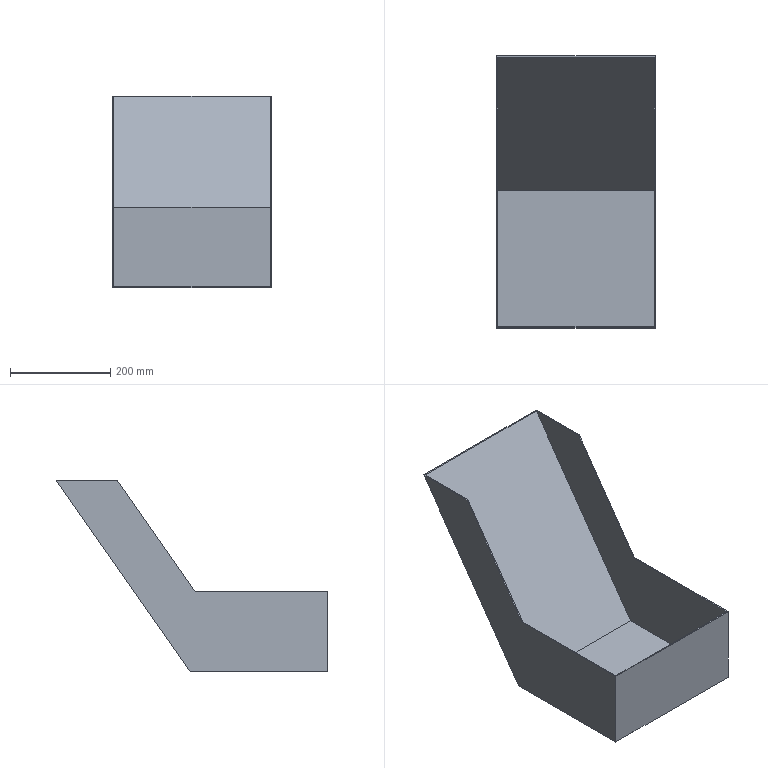Part | STEP file | Tube necking machine_id314_x_t | 1 solid | 14 faces | box 317 x 542.25 x 381.672 mm | volume 881739 mm3 | plane 14
STEP:
#1=CARTESIAN_POINT('',(0.,0.,0.));
#2=DIRECTION('',(0.,0.,1.));
#3=DIRECTION('',(1.,0.,0.));
#4=AXIS2_PLACEMENT_3D('',#1,#2,#3);
#5=CARTESIAN_POINT('',(158.5,-128.618,143.384));
#6=VERTEX_POINT('',#5);
#7=CARTESIAN_POINT('',(158.5,-283.834,-78.288));
#8=VERTEX_POINT('',#7);
#9=CARTESIAN_POINT('',(158.5,-355.705,-180.931));
#10=DIRECTION('',(0.,-0.5736,-0.8192));
#11=VECTOR('',#10,1.);
#12=LINE('',#9,#11);
#13=CARTESIAN_POINT('',(158.5,-355.705,-180.931));
#14=DIRECTION('',(0.,0.8192,-0.5736));
#15=DIRECTION('',(0.,0.5736,0.8192));
#16=AXIS2_PLACEMENT_3D('',#13,#14,#15);
#17=PLANE('',#16);
#18=CARTESIAN_POINT('',(0.,0.));
#19=DIRECTION('',(-1.,0.));
#20=VECTOR('',#19,1.);
#21=LINE('',#18,#20);
#22=(GEOMETRIC_REPRESENTATION_CONTEXT(2)PARAMETRIC_REPRESENTATION_CONTEXT()REPRESENTATION_CONTEXT('',''));
#23=DEFINITIONAL_REPRESENTATION('',(#21),#22);
#24=PCURVE('',#17,#23);
#25=CARTESIAN_POINT('',(158.5,-273.79,-238.288));
#26=DIRECTION('',(1.,0.,0.));
#27=DIRECTION('',(0.,0.,-1.));
#28=AXIS2_PLACEMENT_3D('',#25,#26,#27);
#29=PLANE('',#28);
#30=CARTESIAN_POINT('',(-57.358,-81.915));
#31=DIRECTION('',(0.8192,-0.5736));
#32=VECTOR('',#31,1.);
#33=LINE('',#30,#32);
#34=(GEOMETRIC_REPRESENTATION_CONTEXT(2)PARAMETRIC_REPRESENTATION_CONTEXT()REPRESENTATION_CONTEXT('',''));
#35=DEFINITIONAL_REPRESENTATION('',(#33),#34);
#36=PCURVE('',#29,#35);
#37=SURFACE_CURVE('',#12,(#24,#36),.PCURVE_S1.);
#38=EDGE_CURVE('',#6,#8,#37,.T.);
#39=ORIENTED_EDGE('',*,*,#38,.F.);
#40=CARTESIAN_POINT('',(156.5,-128.618,143.384));
#41=VERTEX_POINT('',#40);
#42=CARTESIAN_POINT('',(158.5,-128.618,143.384));
#43=DIRECTION('',(-1.,0.,0.));
#44=VECTOR('',#43,1.);
#45=LINE('',#42,#44);
#46=CARTESIAN_POINT('',(395.915,0.));
#47=DIRECTION('',(0.,-1.));
#48=VECTOR('',#47,1.);
#49=LINE('',#46,#48);
#50=(GEOMETRIC_REPRESENTATION_CONTEXT(2)PARAMETRIC_REPRESENTATION_CONTEXT()REPRESENTATION_CONTEXT('',''));
#51=DEFINITIONAL_REPRESENTATION('',(#49),#50);
#52=PCURVE('',#17,#51);
#53=CARTESIAN_POINT('',(-158.5,-6.541,143.384));
#54=DIRECTION('',(0.,0.,1.));
#55=DIRECTION('',(1.,0.,0.));
#56=AXIS2_PLACEMENT_3D('',#53,#54,#55);
#57=PLANE('',#56);
#58=CARTESIAN_POINT('',(317.,-122.077));
#59=DIRECTION('',(-1.,0.));
#60=VECTOR('',#59,1.);
#61=LINE('',#58,#60);
#62=(GEOMETRIC_REPRESENTATION_CONTEXT(2)PARAMETRIC_REPRESENTATION_CONTEXT()REPRESENTATION_CONTEXT('',''));
#63=DEFINITIONAL_REPRESENTATION('',(#61),#62);
#64=PCURVE('',#57,#63);
#65=SURFACE_CURVE('',#45,(#52,#64),.PCURVE_S1.);
#66=EDGE_CURVE('',#6,#41,#65,.T.);
#67=ORIENTED_EDGE('',*,*,#66,.T.);
#68=CARTESIAN_POINT('',(156.5,-283.834,-78.288));
#69=VERTEX_POINT('',#68);
#70=CARTESIAN_POINT('',(156.5,-355.705,-180.931));
#71=DIRECTION('',(0.,-0.5736,-0.8192));
#72=VECTOR('',#71,1.);
#73=LINE('',#70,#72);
#74=CARTESIAN_POINT('',(0.,-2.));
#75=DIRECTION('',(-1.,0.));
#76=VECTOR('',#75,1.);
#77=LINE('',#74,#76);
#78=(GEOMETRIC_REPRESENTATION_CONTEXT(2)PARAMETRIC_REPRESENTATION_CONTEXT()REPRESENTATION_CONTEXT('',''));
#79=DEFINITIONAL_REPRESENTATION('',(#77),#78);
#80=PCURVE('',#17,#79);
#81=CARTESIAN_POINT('',(156.5,-273.79,-238.288));
#82=DIRECTION('',(1.,0.,0.));
#83=DIRECTION('',(0.,0.,-1.));
#84=AXIS2_PLACEMENT_3D('',#81,#82,#83);
#85=PLANE('',#84);
#86=CARTESIAN_POINT('',(-57.358,-81.915));
#87=DIRECTION('',(0.8192,-0.5736));
#88=VECTOR('',#87,1.);
#89=LINE('',#86,#88);
#90=(GEOMETRIC_REPRESENTATION_CONTEXT(2)PARAMETRIC_REPRESENTATION_CONTEXT()REPRESENTATION_CONTEXT('',''));
#91=DEFINITIONAL_REPRESENTATION('',(#89),#90);
#92=PCURVE('',#85,#91);
#93=SURFACE_CURVE('',#73,(#80,#92),.PCURVE_S1.);
#94=EDGE_CURVE('',#41,#69,#93,.T.);
#95=ORIENTED_EDGE('',*,*,#94,.T.);
#96=CARTESIAN_POINT('',(158.5,-283.834,-78.288));
#97=DIRECTION('',(-1.,0.,0.));
#98=VECTOR('',#97,1.);
#99=LINE('',#96,#98);
#100=CARTESIAN_POINT('',(125.303,0.));
#101=DIRECTION('',(0.,-1.));
#102=VECTOR('',#101,1.);
#103=LINE('',#100,#102);
#104=(GEOMETRIC_REPRESENTATION_CONTEXT(2)PARAMETRIC_REPRESENTATION_CONTEXT()REPRESENTATION_CONTEXT('',''));
#105=DEFINITIONAL_REPRESENTATION('',(#103),#104);
#106=PCURVE('',#17,#105);
#107=CARTESIAN_POINT('',(158.5,-273.79,-78.288));
#108=DIRECTION('',(0.,0.,-1.));
#109=DIRECTION('',(0.,-1.,0.));
#110=AXIS2_PLACEMENT_3D('',#107,#108,#109);
#111=PLANE('',#110);
#112=CARTESIAN_POINT('',(10.044,0.));
#113=DIRECTION('',(0.,1.));
#114=VECTOR('',#113,1.);
#115=LINE('',#112,#114);
#116=(GEOMETRIC_REPRESENTATION_CONTEXT(2)PARAMETRIC_REPRESENTATION_CONTEXT()REPRESENTATION_CONTEXT('',''));
#117=DEFINITIONAL_REPRESENTATION('',(#115),#116);
#118=PCURVE('',#111,#117);
#119=SURFACE_CURVE('',#99,(#106,#118),.PCURVE_S1.);
#120=EDGE_CURVE('',#8,#69,#119,.T.);
#121=ORIENTED_EDGE('',*,*,#120,.F.);
#122=EDGE_LOOP('',(#39,#67,#95,#121));
#123=FACE_BOUND('',#122,.T.);
#124=ADVANCED_FACE('',(#123),#17,.F.);
#125=CARTESIAN_POINT('',(-156.5,-283.834,-78.288));
#126=VERTEX_POINT('',#125);
#127=CARTESIAN_POINT('',(-156.5,-128.618,143.384));
#128=VERTEX_POINT('',#127);
#129=CARTESIAN_POINT('',(-156.5,-88.456,200.741));
#130=DIRECTION('',(0.,0.5736,0.8192));
#131=VECTOR('',#130,1.);
#132=LINE('',#129,#131);
#133=CARTESIAN_POINT('',(-158.5,-88.456,200.741));
#134=DIRECTION('',(0.,0.8192,-0.5736));
#135=DIRECTION('',(0.,-0.5736,-0.8192));
#136=AXIS2_PLACEMENT_3D('',#133,#134,#135);
#137=PLANE('',#136);
#138=CARTESIAN_POINT('',(0.,-2.));
#139=DIRECTION('',(-1.,0.));
#140=VECTOR('',#139,1.);
#141=LINE('',#138,#140);
#142=(GEOMETRIC_REPRESENTATION_CONTEXT(2)PARAMETRIC_REPRESENTATION_CONTEXT()REPRESENTATION_CONTEXT('',''));
#143=DEFINITIONAL_REPRESENTATION('',(#141),#142);
#144=PCURVE('',#137,#143);
#145=CARTESIAN_POINT('',(-156.5,-6.541,143.384));
#146=DIRECTION('',(-1.,0.,0.));
#147=DIRECTION('',(0.,0.,1.));
#148=AXIS2_PLACEMENT_3D('',#145,#146,#147);
#149=PLANE('',#148);
#150=CARTESIAN_POINT('',(57.358,-81.915));
#151=DIRECTION('',(0.8192,0.5736));
#152=VECTOR('',#151,1.);
#153=LINE('',#150,#152);
#154=(GEOMETRIC_REPRESENTATION_CONTEXT(2)PARAMETRIC_REPRESENTATION_CONTEXT()REPRESENTATION_CONTEXT('',''));
#155=DEFINITIONAL_REPRESENTATION('',(#153),#154);
#156=PCURVE('',#149,#155);
#157=SURFACE_CURVE('',#132,(#144,#156),.PCURVE_S1.);
#158=EDGE_CURVE('',#126,#128,#157,.T.);
#159=ORIENTED_EDGE('',*,*,#158,.T.);
#160=CARTESIAN_POINT('',(-158.5,-128.618,143.384));
#161=VERTEX_POINT('',#160);
#162=CARTESIAN_POINT('',(-158.5,-128.618,143.384));
#163=DIRECTION('',(-1.,0.,0.));
#164=VECTOR('',#163,1.);
#165=LINE('',#162,#164);
#166=CARTESIAN_POINT('',(70.021,0.));
#167=DIRECTION('',(0.,1.));
#168=VECTOR('',#167,1.);
#169=LINE('',#166,#168);
#170=(GEOMETRIC_REPRESENTATION_CONTEXT(2)PARAMETRIC_REPRESENTATION_CONTEXT()REPRESENTATION_CONTEXT('',''));
#171=DEFINITIONAL_REPRESENTATION('',(#169),#170);
#172=PCURVE('',#137,#171);
#173=CARTESIAN_POINT('',(0.,-122.077));
#174=DIRECTION('',(-1.,0.));
#175=VECTOR('',#174,1.);
#176=LINE('',#173,#175);
#177=(GEOMETRIC_REPRESENTATION_CONTEXT(2)PARAMETRIC_REPRESENTATION_CONTEXT()REPRESENTATION_CONTEXT('',''));
#178=DEFINITIONAL_REPRESENTATION('',(#176),#177);
#179=PCURVE('',#57,#178);
#180=SURFACE_CURVE('',#165,(#172,#179),.PCURVE_S1.);
#181=EDGE_CURVE('',#128,#161,#180,.T.);
#182=ORIENTED_EDGE('',*,*,#181,.T.);
#183=CARTESIAN_POINT('',(-158.5,-283.834,-78.288));
#184=VERTEX_POINT('',#183);
#185=CARTESIAN_POINT('',(-158.5,-88.456,200.741));
#186=DIRECTION('',(0.,0.5736,0.8192));
#187=VECTOR('',#186,1.);
#188=LINE('',#185,#187);
#189=CARTESIAN_POINT('',(0.,0.));
#190=DIRECTION('',(-1.,0.));
#191=VECTOR('',#190,1.);
#192=LINE('',#189,#191);
#193=(GEOMETRIC_REPRESENTATION_CONTEXT(2)PARAMETRIC_REPRESENTATION_CONTEXT()REPRESENTATION_CONTEXT('',''));
#194=DEFINITIONAL_REPRESENTATION('',(#192),#193);
#195=PCURVE('',#137,#194);
#196=CARTESIAN_POINT('',(-158.5,-6.541,143.384));
#197=DIRECTION('',(-1.,0.,0.));
#198=DIRECTION('',(0.,0.,1.));
#199=AXIS2_PLACEMENT_3D('',#196,#197,#198);
#200=PLANE('',#199);
#201=CARTESIAN_POINT('',(57.358,-81.915));
#202=DIRECTION('',(0.8192,0.5736));
#203=VECTOR('',#202,1.);
#204=LINE('',#201,#203);
#205=(GEOMETRIC_REPRESENTATION_CONTEXT(2)PARAMETRIC_REPRESENTATION_CONTEXT()REPRESENTATION_CONTEXT('',''));
#206=DEFINITIONAL_REPRESENTATION('',(#204),#205);
#207=PCURVE('',#200,#206);
#208=SURFACE_CURVE('',#188,(#195,#207),.PCURVE_S1.);
#209=EDGE_CURVE('',#184,#161,#208,.T.);
#210=ORIENTED_EDGE('',*,*,#209,.F.);
#211=CARTESIAN_POINT('',(-158.5,-283.834,-78.288));
#212=DIRECTION('',(-1.,0.,0.));
#213=VECTOR('',#212,1.);
#214=LINE('',#211,#213);
#215=CARTESIAN_POINT('',(340.632,0.));
#216=DIRECTION('',(0.,1.));
#217=VECTOR('',#216,1.);
#218=LINE('',#215,#217);
#219=(GEOMETRIC_REPRESENTATION_CONTEXT(2)PARAMETRIC_REPRESENTATION_CONTEXT()REPRESENTATION_CONTEXT('',''));
#220=DEFINITIONAL_REPRESENTATION('',(#218),#219);
#221=PCURVE('',#137,#220);
#222=CARTESIAN_POINT('',(10.044,317.));
#223=DIRECTION('',(0.,1.));
#224=VECTOR('',#223,1.);
#225=LINE('',#222,#224);
#226=(GEOMETRIC_REPRESENTATION_CONTEXT(2)PARAMETRIC_REPRESENTATION_CONTEXT()REPRESENTATION_CONTEXT('',''));
#227=DEFINITIONAL_REPRESENTATION('',(#225),#226);
#228=PCURVE('',#111,#227);
#229=SURFACE_CURVE('',#214,(#221,#228),.PCURVE_S1.);
#230=EDGE_CURVE('',#126,#184,#229,.T.);
#231=ORIENTED_EDGE('',*,*,#230,.F.);
#232=EDGE_LOOP('',(#159,#182,#210,#231));
#233=FACE_BOUND('',#232,.T.);
#234=ADVANCED_FACE('',(#233),#137,.F.);
#235=CARTESIAN_POINT('',(-156.5,-8.982,143.384));
#236=VERTEX_POINT('',#235);
#237=CARTESIAN_POINT('',(-156.5,-6.541,143.384));
#238=DIRECTION('',(0.,1.,0.));
#239=VECTOR('',#238,1.);
#240=LINE('',#237,#239);
#241=CARTESIAN_POINT('',(0.,0.));
#242=DIRECTION('',(0.,1.));
#243=VECTOR('',#242,1.);
#244=LINE('',#241,#243);
#245=(GEOMETRIC_REPRESENTATION_CONTEXT(2)PARAMETRIC_REPRESENTATION_CONTEXT()REPRESENTATION_CONTEXT('',''));
#246=DEFINITIONAL_REPRESENTATION('',(#244),#245);
#247=PCURVE('',#149,#246);
#248=CARTESIAN_POINT('',(2.,0.));
#249=DIRECTION('',(0.,1.));
#250=VECTOR('',#249,1.);
#251=LINE('',#248,#250);
#252=(GEOMETRIC_REPRESENTATION_CONTEXT(2)PARAMETRIC_REPRESENTATION_CONTEXT()REPRESENTATION_CONTEXT('',''));
#253=DEFINITIONAL_REPRESENTATION('',(#251),#252);
#254=PCURVE('',#57,#253);
#255=SURFACE_CURVE('',#240,(#247,#254),.PCURVE_S1.);
#256=EDGE_CURVE('',#128,#236,#255,.T.);
#257=ORIENTED_EDGE('',*,*,#256,.F.);
#258=ORIENTED_EDGE('',*,*,#158,.F.);
#259=CARTESIAN_POINT('',(-156.5,-546.79,-78.288));
#260=VERTEX_POINT('',#259);
#261=CARTESIAN_POINT('',(-156.5,-548.79,-78.288));
#262=DIRECTION('',(0.,-1.,0.));
#263=VECTOR('',#262,1.);
#264=LINE('',#261,#263);
#265=CARTESIAN_POINT('',(-221.672,-542.25));
#266=DIRECTION('',(0.,-1.));
#267=VECTOR('',#266,1.);
#268=LINE('',#265,#267);
#269=(GEOMETRIC_REPRESENTATION_CONTEXT(2)PARAMETRIC_REPRESENTATION_CONTEXT()REPRESENTATION_CONTEXT('',''));
#270=DEFINITIONAL_REPRESENTATION('',(#268),#269);
#271=PCURVE('',#149,#270);
#272=CARTESIAN_POINT('',(275.,315.));
#273=DIRECTION('',(1.,0.));
#274=VECTOR('',#273,1.);
#275=LINE('',#272,#274);
#276=(GEOMETRIC_REPRESENTATION_CONTEXT(2)PARAMETRIC_REPRESENTATION_CONTEXT()REPRESENTATION_CONTEXT('',''));
#277=DEFINITIONAL_REPRESENTATION('',(#275),#276);
#278=PCURVE('',#111,#277);
#279=SURFACE_CURVE('',#264,(#271,#278),.PCURVE_S1.);
#280=EDGE_CURVE('',#126,#260,#279,.T.);
#281=ORIENTED_EDGE('',*,*,#280,.T.);
#282=CARTESIAN_POINT('',(-156.5,-546.79,-236.288));
#283=VERTEX_POINT('',#282);
#284=CARTESIAN_POINT('',(-156.5,-546.79,-238.288));
#285=DIRECTION('',(0.,0.,1.));
#286=VECTOR('',#285,1.);
#287=LINE('',#284,#286);
#288=CARTESIAN_POINT('',(-381.672,-540.25));
#289=DIRECTION('',(1.,0.));
#290=VECTOR('',#289,1.);
#291=LINE('',#288,#290);
#292=(GEOMETRIC_REPRESENTATION_CONTEXT(2)PARAMETRIC_REPRESENTATION_CONTEXT()REPRESENTATION_CONTEXT('',''));
#293=DEFINITIONAL_REPRESENTATION('',(#291),#292);
#294=PCURVE('',#149,#293);
#295=CARTESIAN_POINT('',(241.8,-546.79,-238.288));
#296=DIRECTION('',(0.,-1.,0.));
#297=DIRECTION('',(0.,0.,-1.));
#298=AXIS2_PLACEMENT_3D('',#295,#296,#297);
#299=PLANE('',#298);
#300=CARTESIAN_POINT('',(0.,-398.3));
#301=DIRECTION('',(-1.,0.));
#302=VECTOR('',#301,1.);
#303=LINE('',#300,#302);
#304=(GEOMETRIC_REPRESENTATION_CONTEXT(2)PARAMETRIC_REPRESENTATION_CONTEXT()REPRESENTATION_CONTEXT('',''));
#305=DEFINITIONAL_REPRESENTATION('',(#303),#304);
#306=PCURVE('',#299,#305);
#307=SURFACE_CURVE('',#287,(#294,#306),.PCURVE_S1.);
#308=EDGE_CURVE('',#283,#260,#307,.T.);
#309=ORIENTED_EDGE('',*,*,#308,.F.);
#310=CARTESIAN_POINT('',(-156.5,-274.831,-236.288));
#311=VERTEX_POINT('',#310);
#312=CARTESIAN_POINT('',(-156.5,-273.79,-236.288));
#313=DIRECTION('',(0.,-1.,0.));
#314=VECTOR('',#313,1.);
#315=LINE('',#312,#314);
#316=CARTESIAN_POINT('',(-379.672,-267.25));
#317=DIRECTION('',(0.,-1.));
#318=VECTOR('',#317,1.);
#319=LINE('',#316,#318);
#320=(GEOMETRIC_REPRESENTATION_CONTEXT(2)PARAMETRIC_REPRESENTATION_CONTEXT()REPRESENTATION_CONTEXT('',''));
#321=DEFINITIONAL_REPRESENTATION('',(#319),#320);
#322=PCURVE('',#149,#321);
#323=CARTESIAN_POINT('',(241.8,-273.79,-236.288));
#324=DIRECTION('',(0.,0.,-1.));
#325=DIRECTION('',(-1.,0.,0.));
#326=AXIS2_PLACEMENT_3D('',#323,#324,#325);
#327=PLANE('',#326);
#328=CARTESIAN_POINT('',(398.3,0.));
#329=DIRECTION('',(0.,-1.));
#330=VECTOR('',#329,1.);
#331=LINE('',#328,#330);
#332=(GEOMETRIC_REPRESENTATION_CONTEXT(2)PARAMETRIC_REPRESENTATION_CONTEXT()REPRESENTATION_CONTEXT('',''));
#333=DEFINITIONAL_REPRESENTATION('',(#331),#332);
#334=PCURVE('',#327,#333);
#335=SURFACE_CURVE('',#315,(#322,#334),.PCURVE_S1.);
#336=EDGE_CURVE('',#311,#283,#335,.T.);
#337=ORIENTED_EDGE('',*,*,#336,.F.);
#338=CARTESIAN_POINT('',(-156.5,-8.179,144.531));
#339=DIRECTION('',(0.,-0.5736,-0.8192));
#340=VECTOR('',#339,1.);
#341=LINE('',#338,#340);
#342=CARTESIAN_POINT('',(1.147,-1.638));
#343=DIRECTION('',(-0.8192,-0.5736));
#344=VECTOR('',#343,1.);
#345=LINE('',#342,#344);
#346=(GEOMETRIC_REPRESENTATION_CONTEXT(2)PARAMETRIC_REPRESENTATION_CONTEXT()REPRESENTATION_CONTEXT('',''));
#347=DEFINITIONAL_REPRESENTATION('',(#345),#346);
#348=PCURVE('',#149,#347);
#349=CARTESIAN_POINT('',(241.8,-8.179,144.531));
#350=DIRECTION('',(0.,0.8192,-0.5736));
#351=DIRECTION('',(0.,0.5736,0.8192));
#352=AXIS2_PLACEMENT_3D('',#349,#350,#351);
#353=PLANE('',#352);
#354=CARTESIAN_POINT('',(0.,-398.3));
#355=DIRECTION('',(-1.,0.));
#356=VECTOR('',#355,1.);
#357=LINE('',#354,#356);
#358=(GEOMETRIC_REPRESENTATION_CONTEXT(2)PARAMETRIC_REPRESENTATION_CONTEXT()REPRESENTATION_CONTEXT('',''));
#359=DEFINITIONAL_REPRESENTATION('',(#357),#358);
#360=PCURVE('',#353,#359);
#361=SURFACE_CURVE('',#341,(#348,#360),.PCURVE_S1.);
#362=EDGE_CURVE('',#236,#311,#361,.T.);
#363=ORIENTED_EDGE('',*,*,#362,.F.);
#364=EDGE_LOOP('',(#257,#258,#281,#309,#337,#363));
#365=FACE_BOUND('',#364,.T.);
#366=ADVANCED_FACE('',(#365),#149,.F.);
#367=CARTESIAN_POINT('',(156.5,-8.982,143.384));
#368=VERTEX_POINT('',#367);
#369=CARTESIAN_POINT('',(241.8,-8.982,143.384));
#370=DIRECTION('',(1.,0.,0.));
#371=VECTOR('',#370,1.);
#372=LINE('',#369,#371);
#373=CARTESIAN_POINT('',(-1.4,0.));
#374=DIRECTION('',(0.,1.));
#375=VECTOR('',#374,1.);
#376=LINE('',#373,#375);
#377=(GEOMETRIC_REPRESENTATION_CONTEXT(2)PARAMETRIC_REPRESENTATION_CONTEXT()REPRESENTATION_CONTEXT('',''));
#378=DEFINITIONAL_REPRESENTATION('',(#376),#377);
#379=PCURVE('',#353,#378);
#380=CARTESIAN_POINT('',(400.3,-2.442));
#381=DIRECTION('',(1.,0.));
#382=VECTOR('',#381,1.);
#383=LINE('',#380,#382);
#384=(GEOMETRIC_REPRESENTATION_CONTEXT(2)PARAMETRIC_REPRESENTATION_CONTEXT()REPRESENTATION_CONTEXT('',''));
#385=DEFINITIONAL_REPRESENTATION('',(#383),#384);
#386=PCURVE('',#57,#385);
#387=SURFACE_CURVE('',#372,(#379,#386),.PCURVE_S1.);
#388=EDGE_CURVE('',#236,#368,#387,.T.);
#389=ORIENTED_EDGE('',*,*,#388,.F.);
#390=ORIENTED_EDGE('',*,*,#362,.T.);
#391=CARTESIAN_POINT('',(156.5,-274.831,-236.288));
#392=VERTEX_POINT('',#391);
#393=CARTESIAN_POINT('',(241.8,-274.831,-236.288));
#394=DIRECTION('',(-1.,0.,0.));
#395=VECTOR('',#394,1.);
#396=LINE('',#393,#395);
#397=CARTESIAN_POINT('',(-464.894,0.));
#398=DIRECTION('',(0.,-1.));
#399=VECTOR('',#398,1.);
#400=LINE('',#397,#399);
#401=(GEOMETRIC_REPRESENTATION_CONTEXT(2)PARAMETRIC_REPRESENTATION_CONTEXT()REPRESENTATION_CONTEXT('',''));
#402=DEFINITIONAL_REPRESENTATION('',(#400),#401);
#403=PCURVE('',#353,#402);
#404=CARTESIAN_POINT('',(0.,-1.041));
#405=DIRECTION('',(1.,0.));
#406=VECTOR('',#405,1.);
#407=LINE('',#404,#406);
#408=(GEOMETRIC_REPRESENTATION_CONTEXT(2)PARAMETRIC_REPRESENTATION_CONTEXT()REPRESENTATION_CONTEXT('',''));
#409=DEFINITIONAL_REPRESENTATION('',(#407),#408);
#410=PCURVE('',#327,#409);
#411=SURFACE_CURVE('',#396,(#403,#410),.PCURVE_S1.);
#412=EDGE_CURVE('',#392,#311,#411,.T.);
#413=ORIENTED_EDGE('',*,*,#412,.F.);
#414=CARTESIAN_POINT('',(156.5,-8.179,144.531));
#415=DIRECTION('',(0.,-0.5736,-0.8192));
#416=VECTOR('',#415,1.);
#417=LINE('',#414,#416);
#418=CARTESIAN_POINT('',(0.,-85.3));
#419=DIRECTION('',(-1.,0.));
#420=VECTOR('',#419,1.);
#421=LINE('',#418,#420);
#422=(GEOMETRIC_REPRESENTATION_CONTEXT(2)PARAMETRIC_REPRESENTATION_CONTEXT()REPRESENTATION_CONTEXT('',''));
#423=DEFINITIONAL_REPRESENTATION('',(#421),#422);
#424=PCURVE('',#353,#423);
#425=CARTESIAN_POINT('',(-382.819,265.611));
#426=DIRECTION('',(0.8192,-0.5736));
#427=VECTOR('',#426,1.);
#428=LINE('',#425,#427);
#429=(GEOMETRIC_REPRESENTATION_CONTEXT(2)PARAMETRIC_REPRESENTATION_CONTEXT()REPRESENTATION_CONTEXT('',''));
#430=DEFINITIONAL_REPRESENTATION('',(#428),#429);
#431=PCURVE('',#85,#430);
#432=SURFACE_CURVE('',#417,(#424,#431),.PCURVE_S1.);
#433=EDGE_CURVE('',#368,#392,#432,.T.);
#434=ORIENTED_EDGE('',*,*,#433,.F.);
#435=EDGE_LOOP('',(#389,#390,#413,#434));
#436=FACE_BOUND('',#435,.T.);
#437=ADVANCED_FACE('',(#436),#353,.F.);
#438=CARTESIAN_POINT('',(156.5,-273.79,143.384));
#439=DIRECTION('',(0.,-1.,0.));
#440=VECTOR('',#439,1.);
#441=LINE('',#438,#440);
#442=CARTESIAN_POINT('',(-381.672,0.));
#443=DIRECTION('',(0.,-1.));
#444=VECTOR('',#443,1.);
#445=LINE('',#442,#444);
#446=(GEOMETRIC_REPRESENTATION_CONTEXT(2)PARAMETRIC_REPRESENTATION_CONTEXT()REPRESENTATION_CONTEXT('',''));
#447=DEFINITIONAL_REPRESENTATION('',(#445),#446);
#448=PCURVE('',#85,#447);
#449=CARTESIAN_POINT('',(315.,-267.25));
#450=DIRECTION('',(0.,-1.));
#451=VECTOR('',#450,1.);
#452=LINE('',#449,#451);
#453=(GEOMETRIC_REPRESENTATION_CONTEXT(2)PARAMETRIC_REPRESENTATION_CONTEXT()REPRESENTATION_CONTEXT('',''));
#454=DEFINITIONAL_REPRESENTATION('',(#452),#453);
#455=PCURVE('',#57,#454);
#456=SURFACE_CURVE('',#441,(#448,#455),.PCURVE_S1.);
#457=EDGE_CURVE('',#368,#41,#456,.T.);
#458=ORIENTED_EDGE('',*,*,#457,.F.);
#459=ORIENTED_EDGE('',*,*,#433,.T.);
#460=CARTESIAN_POINT('',(156.5,-546.79,-236.288));
#461=VERTEX_POINT('',#460);
#462=CARTESIAN_POINT('',(156.5,-273.79,-236.288));
#463=DIRECTION('',(0.,-1.,0.));
#464=VECTOR('',#463,1.);
#465=LINE('',#462,#464);
#466=CARTESIAN_POINT('',(-2.,0.));
#467=DIRECTION('',(0.,-1.));
#468=VECTOR('',#467,1.);
#469=LINE('',#466,#468);
#470=(GEOMETRIC_REPRESENTATION_CONTEXT(2)PARAMETRIC_REPRESENTATION_CONTEXT()REPRESENTATION_CONTEXT('',''));
#471=DEFINITIONAL_REPRESENTATION('',(#469),#470);
#472=PCURVE('',#85,#471);
#473=CARTESIAN_POINT('',(85.3,0.));
#474=DIRECTION('',(0.,-1.));
#475=VECTOR('',#474,1.);
#476=LINE('',#473,#475);
#477=(GEOMETRIC_REPRESENTATION_CONTEXT(2)PARAMETRIC_REPRESENTATION_CONTEXT()REPRESENTATION_CONTEXT('',''));
#478=DEFINITIONAL_REPRESENTATION('',(#476),#477);
#479=PCURVE('',#327,#478);
#480=SURFACE_CURVE('',#465,(#472,#479),.PCURVE_S1.);
#481=EDGE_CURVE('',#392,#461,#480,.T.);
#482=ORIENTED_EDGE('',*,*,#481,.T.);
#483=CARTESIAN_POINT('',(156.5,-546.79,-78.288));
#484=VERTEX_POINT('',#483);
#485=CARTESIAN_POINT('',(156.5,-546.79,-238.288));
#486=DIRECTION('',(0.,0.,-1.));
#487=VECTOR('',#486,1.);
#488=LINE('',#485,#487);
#489=CARTESIAN_POINT('',(0.,-273.));
#490=DIRECTION('',(1.,0.));
#491=VECTOR('',#490,1.);
#492=LINE('',#489,#491);
#493=(GEOMETRIC_REPRESENTATION_CONTEXT(2)PARAMETRIC_REPRESENTATION_CONTEXT()REPRESENTATION_CONTEXT('',''));
#494=DEFINITIONAL_REPRESENTATION('',(#492),#493);
#495=PCURVE('',#85,#494);
#496=CARTESIAN_POINT('',(0.,-85.3));
#497=DIRECTION('',(1.,0.));
#498=VECTOR('',#497,1.);
#499=LINE('',#496,#498);
#500=(GEOMETRIC_REPRESENTATION_CONTEXT(2)PARAMETRIC_REPRESENTATION_CONTEXT()REPRESENTATION_CONTEXT('',''));
#501=DEFINITIONAL_REPRESENTATION('',(#499),#500);
#502=PCURVE('',#299,#501);
#503=SURFACE_CURVE('',#488,(#495,#502),.PCURVE_S1.);
#504=EDGE_CURVE('',#484,#461,#503,.T.);
#505=ORIENTED_EDGE('',*,*,#504,.F.);
#506=CARTESIAN_POINT('',(156.5,-273.79,-78.288));
#507=DIRECTION('',(0.,1.,0.));
#508=VECTOR('',#507,1.);
#509=LINE('',#506,#508);
#510=CARTESIAN_POINT('',(-160.,0.));
#511=DIRECTION('',(0.,1.));
#512=VECTOR('',#511,1.);
#513=LINE('',#510,#512);
#514=(GEOMETRIC_REPRESENTATION_CONTEXT(2)PARAMETRIC_REPRESENTATION_CONTEXT()REPRESENTATION_CONTEXT('',''));
#515=DEFINITIONAL_REPRESENTATION('',(#513),#514);
#516=PCURVE('',#85,#515);
#517=CARTESIAN_POINT('',(0.,2.));
#518=DIRECTION('',(-1.,0.));
#519=VECTOR('',#518,1.);
#520=LINE('',#517,#519);
#521=(GEOMETRIC_REPRESENTATION_CONTEXT(2)PARAMETRIC_REPRESENTATION_CONTEXT()REPRESENTATION_CONTEXT('',''));
#522=DEFINITIONAL_REPRESENTATION('',(#520),#521);
#523=PCURVE('',#111,#522);
#524=SURFACE_CURVE('',#509,(#516,#523),.PCURVE_S1.);
#525=EDGE_CURVE('',#484,#69,#524,.T.);
#526=ORIENTED_EDGE('',*,*,#525,.T.);
#527=ORIENTED_EDGE('',*,*,#94,.F.);
#528=EDGE_LOOP('',(#458,#459,#482,#505,#526,#527));
#529=FACE_BOUND('',#528,.T.);
#530=ADVANCED_FACE('',(#529),#85,.F.);
#531=ORIENTED_EDGE('',*,*,#209,.T.);
#532=CARTESIAN_POINT('',(-158.5,-6.541,143.384));
#533=VERTEX_POINT('',#532);
#534=CARTESIAN_POINT('',(-158.5,-6.541,143.384));
#535=DIRECTION('',(0.,1.,0.));
#536=VECTOR('',#535,1.);
#537=LINE('',#534,#536);
#538=CARTESIAN_POINT('',(0.,0.));
#539=DIRECTION('',(0.,1.));
#540=VECTOR('',#539,1.);
#541=LINE('',#538,#540);
#542=(GEOMETRIC_REPRESENTATION_CONTEXT(2)PARAMETRIC_REPRESENTATION_CONTEXT()REPRESENTATION_CONTEXT('',''));
#543=DEFINITIONAL_REPRESENTATION('',(#541),#542);
#544=PCURVE('',#200,#543);
#545=CARTESIAN_POINT('',(0.,0.));
#546=DIRECTION('',(0.,1.));
#547=VECTOR('',#546,1.);
#548=LINE('',#545,#547);
#549=(GEOMETRIC_REPRESENTATION_CONTEXT(2)PARAMETRIC_REPRESENTATION_CONTEXT()REPRESENTATION_CONTEXT('',''));
#550=DEFINITIONAL_REPRESENTATION('',(#548),#549);
#551=PCURVE('',#57,#550);
#552=SURFACE_CURVE('',#537,(#544,#551),.PCURVE_S1.);
#553=EDGE_CURVE('',#161,#533,#552,.T.);
#554=ORIENTED_EDGE('',*,*,#553,.T.);
#555=CARTESIAN_POINT('',(-158.5,-273.79,-238.288));
#556=VERTEX_POINT('',#555);
#557=CARTESIAN_POINT('',(-158.5,-6.541,143.384));
#558=DIRECTION('',(0.,-0.5736,-0.8192));
#559=VECTOR('',#558,1.);
#560=LINE('',#557,#559);
#561=CARTESIAN_POINT('',(0.,0.));
#562=DIRECTION('',(-0.8192,-0.5736));
#563=VECTOR('',#562,1.);
#564=LINE('',#561,#563);
#565=(GEOMETRIC_REPRESENTATION_CONTEXT(2)PARAMETRIC_REPRESENTATION_CONTEXT()REPRESENTATION_CONTEXT('',''));
#566=DEFINITIONAL_REPRESENTATION('',(#564),#565);
#567=PCURVE('',#200,#566);
#568=CARTESIAN_POINT('',(241.8,-6.541,143.384));
#569=DIRECTION('',(0.,0.8192,-0.5736));
#570=DIRECTION('',(0.,0.5736,0.8192));
#571=AXIS2_PLACEMENT_3D('',#568,#569,#570);
#572=PLANE('',#571);
#573=CARTESIAN_POINT('',(0.,-400.3));
#574=DIRECTION('',(-1.,0.));
#575=VECTOR('',#574,1.);
#576=LINE('',#573,#575);
#577=(GEOMETRIC_REPRESENTATION_CONTEXT(2)PARAMETRIC_REPRESENTATION_CONTEXT()REPRESENTATION_CONTEXT('',''));
#578=DEFINITIONAL_REPRESENTATION('',(#576),#577);
#579=PCURVE('',#572,#578);
#580=SURFACE_CURVE('',#560,(#567,#579),.PCURVE_S1.);
#581=EDGE_CURVE('',#533,#556,#580,.T.);
#582=ORIENTED_EDGE('',*,*,#581,.T.);
#583=CARTESIAN_POINT('',(-158.5,-548.79,-238.288));
#584=VERTEX_POINT('',#583);
#585=CARTESIAN_POINT('',(-158.5,-411.29,-238.288));
#586=DIRECTION('',(0.,1.,0.));
#587=VECTOR('',#586,1.);
#588=LINE('',#585,#587);
#589=CARTESIAN_POINT('',(-381.672,-404.75));
#590=DIRECTION('',(0.,1.));
#591=VECTOR('',#590,1.);
#592=LINE('',#589,#591);
#593=(GEOMETRIC_REPRESENTATION_CONTEXT(2)PARAMETRIC_REPRESENTATION_CONTEXT()REPRESENTATION_CONTEXT('',''));
#594=DEFINITIONAL_REPRESENTATION('',(#592),#593);
#595=PCURVE('',#200,#594);
#596=CARTESIAN_POINT('',(241.8,-273.79,-238.288));
#597=DIRECTION('',(0.,0.,-1.));
#598=DIRECTION('',(-1.,0.,0.));
#599=AXIS2_PLACEMENT_3D('',#596,#597,#598);
#600=PLANE('',#599);
#601=CARTESIAN_POINT('',(400.3,-137.5));
#602=DIRECTION('',(0.,1.));
#603=VECTOR('',#602,1.);
#604=LINE('',#601,#603);
#605=(GEOMETRIC_REPRESENTATION_CONTEXT(2)PARAMETRIC_REPRESENTATION_CONTEXT()REPRESENTATION_CONTEXT('',''));
#606=DEFINITIONAL_REPRESENTATION('',(#604),#605);
#607=PCURVE('',#600,#606);
#608=SURFACE_CURVE('',#588,(#595,#607),.PCURVE_S1.);
#609=EDGE_CURVE('',#584,#556,#608,.T.);
#610=ORIENTED_EDGE('',*,*,#609,.F.);
#611=CARTESIAN_POINT('',(-158.5,-548.79,-78.288));
#612=VERTEX_POINT('',#611);
#613=CARTESIAN_POINT('',(-158.5,-548.79,-155.788));
#614=DIRECTION('',(0.,0.,-1.));
#615=VECTOR('',#614,1.);
#616=LINE('',#613,#615);
#617=CARTESIAN_POINT('',(-299.172,-542.25));
#618=DIRECTION('',(-1.,0.));
#619=VECTOR('',#618,1.);
#620=LINE('',#617,#619);
#621=(GEOMETRIC_REPRESENTATION_CONTEXT(2)PARAMETRIC_REPRESENTATION_CONTEXT()REPRESENTATION_CONTEXT('',''));
#622=DEFINITIONAL_REPRESENTATION('',(#620),#621);
#623=PCURVE('',#200,#622);
#624=CARTESIAN_POINT('',(241.8,-548.79,-238.288));
#625=DIRECTION('',(0.,-1.,0.));
#626=DIRECTION('',(0.,0.,-1.));
#627=AXIS2_PLACEMENT_3D('',#624,#625,#626);
#628=PLANE('',#627);
#629=CARTESIAN_POINT('',(-82.5,-400.3));
#630=DIRECTION('',(1.,0.));
#631=VECTOR('',#630,1.);
#632=LINE('',#629,#631);
#633=(GEOMETRIC_REPRESENTATION_CONTEXT(2)PARAMETRIC_REPRESENTATION_CONTEXT()REPRESENTATION_CONTEXT('',''));
#634=DEFINITIONAL_REPRESENTATION('',(#632),#633);
#635=PCURVE('',#628,#634);
#636=SURFACE_CURVE('',#616,(#623,#635),.PCURVE_S1.);
#637=EDGE_CURVE('',#612,#584,#636,.T.);
#638=ORIENTED_EDGE('',*,*,#637,.F.);
#639=CARTESIAN_POINT('',(-158.5,-6.541,-78.288));
#640=DIRECTION('',(0.,1.,0.));
#641=VECTOR('',#640,1.);
#642=LINE('',#639,#641);
#643=CARTESIAN_POINT('',(-221.672,0.));
#644=DIRECTION('',(0.,1.));
#645=VECTOR('',#644,1.);
#646=LINE('',#643,#645);
#647=(GEOMETRIC_REPRESENTATION_CONTEXT(2)PARAMETRIC_REPRESENTATION_CONTEXT()REPRESENTATION_CONTEXT('',''));
#648=DEFINITIONAL_REPRESENTATION('',(#646),#647);
#649=PCURVE('',#200,#648);
#650=CARTESIAN_POINT('',(-267.25,317.));
#651=DIRECTION('',(-1.,0.));
#652=VECTOR('',#651,1.);
#653=LINE('',#650,#652);
#654=(GEOMETRIC_REPRESENTATION_CONTEXT(2)PARAMETRIC_REPRESENTATION_CONTEXT()REPRESENTATION_CONTEXT('',''));
#655=DEFINITIONAL_REPRESENTATION('',(#653),#654);
#656=PCURVE('',#111,#655);
#657=SURFACE_CURVE('',#642,(#649,#656),.PCURVE_S1.);
#658=EDGE_CURVE('',#612,#184,#657,.T.);
#659=ORIENTED_EDGE('',*,*,#658,.T.);
#660=EDGE_LOOP('',(#531,#554,#582,#610,#638,#659));
#661=FACE_BOUND('',#660,.T.);
#662=ADVANCED_FACE('',(#661),#200,.T.);
#663=CARTESIAN_POINT('',(158.5,-6.541,143.384));
#664=VERTEX_POINT('',#663);
#665=CARTESIAN_POINT('',(158.5,-273.79,-238.288));
#666=VERTEX_POINT('',#665);
#667=CARTESIAN_POINT('',(158.5,-140.165,-47.452));
#668=DIRECTION('',(0.,-0.5736,-0.8192));
#669=VECTOR('',#668,1.);
#670=LINE('',#667,#669);
#671=CARTESIAN_POINT('',(-190.836,133.625));
#672=DIRECTION('',(0.8192,-0.5736));
#673=VECTOR('',#672,1.);
#674=LINE('',#671,#673);
#675=(GEOMETRIC_REPRESENTATION_CONTEXT(2)PARAMETRIC_REPRESENTATION_CONTEXT()REPRESENTATION_CONTEXT('',''));
#676=DEFINITIONAL_REPRESENTATION('',(#674),#675);
#677=PCURVE('',#29,#676);
#678=CARTESIAN_POINT('',(-232.968,-83.3));
#679=DIRECTION('',(-1.,0.));
#680=VECTOR('',#679,1.);
#681=LINE('',#678,#680);
#682=(GEOMETRIC_REPRESENTATION_CONTEXT(2)PARAMETRIC_REPRESENTATION_CONTEXT()REPRESENTATION_CONTEXT('',''));
#683=DEFINITIONAL_REPRESENTATION('',(#681),#682);
#684=PCURVE('',#572,#683);
#685=SURFACE_CURVE('',#670,(#677,#684),.PCURVE_S1.);
#686=EDGE_CURVE('',#664,#666,#685,.T.);
#687=ORIENTED_EDGE('',*,*,#686,.F.);
#688=CARTESIAN_POINT('',(158.5,-273.79,143.384));
#689=DIRECTION('',(0.,-1.,0.));
#690=VECTOR('',#689,1.);
#691=LINE('',#688,#690);
#692=CARTESIAN_POINT('',(-381.672,0.));
#693=DIRECTION('',(0.,-1.));
#694=VECTOR('',#693,1.);
#695=LINE('',#692,#694);
#696=(GEOMETRIC_REPRESENTATION_CONTEXT(2)PARAMETRIC_REPRESENTATION_CONTEXT()REPRESENTATION_CONTEXT('',''));
#697=DEFINITIONAL_REPRESENTATION('',(#695),#696);
#698=PCURVE('',#29,#697);
#699=CARTESIAN_POINT('',(317.,-267.25));
#700=DIRECTION('',(0.,-1.));
#701=VECTOR('',#700,1.);
#702=LINE('',#699,#701);
#703=(GEOMETRIC_REPRESENTATION_CONTEXT(2)PARAMETRIC_REPRESENTATION_CONTEXT()REPRESENTATION_CONTEXT('',''));
#704=DEFINITIONAL_REPRESENTATION('',(#702),#703);
#705=PCURVE('',#57,#704);
#706=SURFACE_CURVE('',#691,(#698,#705),.PCURVE_S1.);
#707=EDGE_CURVE('',#664,#6,#706,.T.);
#708=ORIENTED_EDGE('',*,*,#707,.T.);
#709=ORIENTED_EDGE('',*,*,#38,.T.);
#710=CARTESIAN_POINT('',(158.5,-548.79,-78.288));
#711=VERTEX_POINT('',#710);
#712=CARTESIAN_POINT('',(158.5,-273.79,-78.288));
#713=DIRECTION('',(0.,1.,0.));
#714=VECTOR('',#713,1.);
#715=LINE('',#712,#714);
#716=CARTESIAN_POINT('',(-160.,0.));
#717=DIRECTION('',(0.,1.));
#718=VECTOR('',#717,1.);
#719=LINE('',#716,#718);
#720=(GEOMETRIC_REPRESENTATION_CONTEXT(2)PARAMETRIC_REPRESENTATION_CONTEXT()REPRESENTATION_CONTEXT('',''));
#721=DEFINITIONAL_REPRESENTATION('',(#719),#720);
#722=PCURVE('',#29,#721);
#723=CARTESIAN_POINT('',(0.,0.));
#724=DIRECTION('',(-1.,0.));
#725=VECTOR('',#724,1.);
#726=LINE('',#723,#725);
#727=(GEOMETRIC_REPRESENTATION_CONTEXT(2)PARAMETRIC_REPRESENTATION_CONTEXT()REPRESENTATION_CONTEXT('',''));
#728=DEFINITIONAL_REPRESENTATION('',(#726),#727);
#729=PCURVE('',#111,#728);
#730=SURFACE_CURVE('',#715,(#722,#729),.PCURVE_S1.);
#731=EDGE_CURVE('',#711,#8,#730,.T.);
#732=ORIENTED_EDGE('',*,*,#731,.F.);
#733=CARTESIAN_POINT('',(158.5,-548.79,-238.288));
#734=VERTEX_POINT('',#733);
#735=CARTESIAN_POINT('',(158.5,-548.79,-155.788));
#736=DIRECTION('',(0.,0.,1.));
#737=VECTOR('',#736,1.);
#738=LINE('',#735,#737);
#739=CARTESIAN_POINT('',(-82.5,-275.));
#740=DIRECTION('',(-1.,0.));
#741=VECTOR('',#740,1.);
#742=LINE('',#739,#741);
#743=(GEOMETRIC_REPRESENTATION_CONTEXT(2)PARAMETRIC_REPRESENTATION_CONTEXT()REPRESENTATION_CONTEXT('',''));
#744=DEFINITIONAL_REPRESENTATION('',(#742),#743);
#745=PCURVE('',#29,#744);
#746=CARTESIAN_POINT('',(-82.5,-83.3));
#747=DIRECTION('',(-1.,0.));
#748=VECTOR('',#747,1.);
#749=LINE('',#746,#748);
#750=(GEOMETRIC_REPRESENTATION_CONTEXT(2)PARAMETRIC_REPRESENTATION_CONTEXT()REPRESENTATION_CONTEXT('',''));
#751=DEFINITIONAL_REPRESENTATION('',(#749),#750);
#752=PCURVE('',#628,#751);
#753=SURFACE_CURVE('',#738,(#745,#752),.PCURVE_S1.);
#754=EDGE_CURVE('',#734,#711,#753,.T.);
#755=ORIENTED_EDGE('',*,*,#754,.F.);
#756=CARTESIAN_POINT('',(158.5,-411.29,-238.288));
#757=DIRECTION('',(0.,-1.,0.));
#758=VECTOR('',#757,1.);
#759=LINE('',#756,#758);
#760=CARTESIAN_POINT('',(0.,-137.5));
#761=DIRECTION('',(0.,-1.));
#762=VECTOR('',#761,1.);
#763=LINE('',#760,#762);
#764=(GEOMETRIC_REPRESENTATION_CONTEXT(2)PARAMETRIC_REPRESENTATION_CONTEXT()REPRESENTATION_CONTEXT('',''));
#765=DEFINITIONAL_REPRESENTATION('',(#763),#764);
#766=PCURVE('',#29,#765);
#767=CARTESIAN_POINT('',(83.3,-137.5));
#768=DIRECTION('',(0.,-1.));
#769=VECTOR('',#768,1.);
#770=LINE('',#767,#769);
#771=(GEOMETRIC_REPRESENTATION_CONTEXT(2)PARAMETRIC_REPRESENTATION_CONTEXT()REPRESENTATION_CONTEXT('',''));
#772=DEFINITIONAL_REPRESENTATION('',(#770),#771);
#773=PCURVE('',#600,#772);
#774=SURFACE_CURVE('',#759,(#766,#773),.PCURVE_S1.);
#775=EDGE_CURVE('',#666,#734,#774,.T.);
#776=ORIENTED_EDGE('',*,*,#775,.F.);
#777=EDGE_LOOP('',(#687,#708,#709,#732,#755,#776));
#778=FACE_BOUND('',#777,.T.);
#779=ADVANCED_FACE('',(#778),#29,.T.);
#780=ORIENTED_EDGE('',*,*,#658,.F.);
#781=CARTESIAN_POINT('',(241.8,-548.79,-78.288));
#782=DIRECTION('',(-1.,0.,0.));
#783=VECTOR('',#782,1.);
#784=LINE('',#781,#783);
#785=CARTESIAN_POINT('',(275.,-83.3));
#786=DIRECTION('',(0.,1.));
#787=VECTOR('',#786,1.);
#788=LINE('',#785,#787);
#789=(GEOMETRIC_REPRESENTATION_CONTEXT(2)PARAMETRIC_REPRESENTATION_CONTEXT()REPRESENTATION_CONTEXT('',''));
#790=DEFINITIONAL_REPRESENTATION('',(#788),#789);
#791=PCURVE('',#111,#790);
#792=CARTESIAN_POINT('',(-160.,0.));
#793=DIRECTION('',(0.,-1.));
#794=VECTOR('',#793,1.);
#795=LINE('',#792,#794);
#796=(GEOMETRIC_REPRESENTATION_CONTEXT(2)PARAMETRIC_REPRESENTATION_CONTEXT()REPRESENTATION_CONTEXT('',''));
#797=DEFINITIONAL_REPRESENTATION('',(#795),#796);
#798=PCURVE('',#628,#797);
#799=SURFACE_CURVE('',#784,(#791,#798),.PCURVE_S1.);
#800=EDGE_CURVE('',#711,#612,#799,.T.);
#801=ORIENTED_EDGE('',*,*,#800,.F.);
#802=ORIENTED_EDGE('',*,*,#731,.T.);
#803=ORIENTED_EDGE('',*,*,#120,.T.);
#804=ORIENTED_EDGE('',*,*,#525,.F.);
#805=CARTESIAN_POINT('',(241.8,-546.79,-78.288));
#806=DIRECTION('',(-1.,0.,0.));
#807=VECTOR('',#806,1.);
#808=LINE('',#805,#807);
#809=CARTESIAN_POINT('',(273.,-83.3));
#810=DIRECTION('',(0.,1.));
#811=VECTOR('',#810,1.);
#812=LINE('',#809,#811);
#813=(GEOMETRIC_REPRESENTATION_CONTEXT(2)PARAMETRIC_REPRESENTATION_CONTEXT()REPRESENTATION_CONTEXT('',''));
#814=DEFINITIONAL_REPRESENTATION('',(#812),#813);
#815=PCURVE('',#111,#814);
#816=CARTESIAN_POINT('',(-160.,0.));
#817=DIRECTION('',(0.,-1.));
#818=VECTOR('',#817,1.);
#819=LINE('',#816,#818);
#820=(GEOMETRIC_REPRESENTATION_CONTEXT(2)PARAMETRIC_REPRESENTATION_CONTEXT()REPRESENTATION_CONTEXT('',''));
#821=DEFINITIONAL_REPRESENTATION('',(#819),#820);
#822=PCURVE('',#299,#821);
#823=SURFACE_CURVE('',#808,(#815,#822),.PCURVE_S1.);
#824=EDGE_CURVE('',#484,#260,#823,.T.);
#825=ORIENTED_EDGE('',*,*,#824,.T.);
#826=ORIENTED_EDGE('',*,*,#280,.F.);
#827=ORIENTED_EDGE('',*,*,#230,.T.);
#828=EDGE_LOOP('',(#780,#801,#802,#803,#804,#825,#826,#827));
#829=FACE_BOUND('',#828,.T.);
#830=ADVANCED_FACE('',(#829),#111,.F.);
#831=ORIENTED_EDGE('',*,*,#308,.T.);
#832=ORIENTED_EDGE('',*,*,#824,.F.);
#833=ORIENTED_EDGE('',*,*,#504,.T.);
#834=CARTESIAN_POINT('',(241.8,-546.79,-236.288));
#835=DIRECTION('',(-1.,0.,0.));
#836=VECTOR('',#835,1.);
#837=LINE('',#834,#836);
#838=CARTESIAN_POINT('',(-2.,0.));
#839=DIRECTION('',(0.,-1.));
#840=VECTOR('',#839,1.);
#841=LINE('',#838,#840);
#842=(GEOMETRIC_REPRESENTATION_CONTEXT(2)PARAMETRIC_REPRESENTATION_CONTEXT()REPRESENTATION_CONTEXT('',''));
#843=DEFINITIONAL_REPRESENTATION('',(#841),#842);
#844=PCURVE('',#299,#843);
#845=CARTESIAN_POINT('',(0.,-273.));
#846=DIRECTION('',(1.,0.));
#847=VECTOR('',#846,1.);
#848=LINE('',#845,#847);
#849=(GEOMETRIC_REPRESENTATION_CONTEXT(2)PARAMETRIC_REPRESENTATION_CONTEXT()REPRESENTATION_CONTEXT('',''));
#850=DEFINITIONAL_REPRESENTATION('',(#848),#849);
#851=PCURVE('',#327,#850);
#852=SURFACE_CURVE('',#837,(#844,#851),.PCURVE_S1.);
#853=EDGE_CURVE('',#461,#283,#852,.T.);
#854=ORIENTED_EDGE('',*,*,#853,.T.);
#855=EDGE_LOOP('',(#831,#832,#833,#854));
#856=FACE_BOUND('',#855,.T.);
#857=ADVANCED_FACE('',(#856),#299,.F.);
#858=ORIENTED_EDGE('',*,*,#336,.T.);
#859=ORIENTED_EDGE('',*,*,#853,.F.);
#860=ORIENTED_EDGE('',*,*,#481,.F.);
#861=ORIENTED_EDGE('',*,*,#412,.T.);
#862=EDGE_LOOP('',(#858,#859,#860,#861));
#863=FACE_BOUND('',#862,.T.);
#864=ADVANCED_FACE('',(#863),#327,.F.);
#865=ORIENTED_EDGE('',*,*,#637,.T.);
#866=CARTESIAN_POINT('',(241.8,-548.79,-238.288));
#867=DIRECTION('',(-1.,0.,0.));
#868=VECTOR('',#867,1.);
#869=LINE('',#866,#868);
#870=CARTESIAN_POINT('',(0.,0.));
#871=DIRECTION('',(0.,-1.));
#872=VECTOR('',#871,1.);
#873=LINE('',#870,#872);
#874=(GEOMETRIC_REPRESENTATION_CONTEXT(2)PARAMETRIC_REPRESENTATION_CONTEXT()REPRESENTATION_CONTEXT('',''));
#875=DEFINITIONAL_REPRESENTATION('',(#873),#874);
#876=PCURVE('',#628,#875);
#877=CARTESIAN_POINT('',(0.,-275.));
#878=DIRECTION('',(1.,0.));
#879=VECTOR('',#878,1.);
#880=LINE('',#877,#879);
#881=(GEOMETRIC_REPRESENTATION_CONTEXT(2)PARAMETRIC_REPRESENTATION_CONTEXT()REPRESENTATION_CONTEXT('',''));
#882=DEFINITIONAL_REPRESENTATION('',(#880),#881);
#883=PCURVE('',#600,#882);
#884=SURFACE_CURVE('',#869,(#876,#883),.PCURVE_S1.);
#885=EDGE_CURVE('',#734,#584,#884,.T.);
#886=ORIENTED_EDGE('',*,*,#885,.F.);
#887=ORIENTED_EDGE('',*,*,#754,.T.);
#888=ORIENTED_EDGE('',*,*,#800,.T.);
#889=EDGE_LOOP('',(#865,#886,#887,#888));
#890=FACE_BOUND('',#889,.T.);
#891=ADVANCED_FACE('',(#890),#628,.T.);
#892=ORIENTED_EDGE('',*,*,#609,.T.);
#893=CARTESIAN_POINT('',(241.8,-273.79,-238.288));
#894=DIRECTION('',(-1.,0.,0.));
#895=VECTOR('',#894,1.);
#896=LINE('',#893,#895);
#897=CARTESIAN_POINT('',(0.,0.));
#898=DIRECTION('',(1.,0.));
#899=VECTOR('',#898,1.);
#900=LINE('',#897,#899);
#901=(GEOMETRIC_REPRESENTATION_CONTEXT(2)PARAMETRIC_REPRESENTATION_CONTEXT()REPRESENTATION_CONTEXT('',''));
#902=DEFINITIONAL_REPRESENTATION('',(#900),#901);
#903=PCURVE('',#600,#902);
#904=CARTESIAN_POINT('',(-465.935,0.));
#905=DIRECTION('',(0.,-1.));
#906=VECTOR('',#905,1.);
#907=LINE('',#904,#906);
#908=(GEOMETRIC_REPRESENTATION_CONTEXT(2)PARAMETRIC_REPRESENTATION_CONTEXT()REPRESENTATION_CONTEXT('',''));
#909=DEFINITIONAL_REPRESENTATION('',(#907),#908);
#910=PCURVE('',#572,#909);
#911=SURFACE_CURVE('',#896,(#903,#910),.PCURVE_S1.);
#912=EDGE_CURVE('',#666,#556,#911,.T.);
#913=ORIENTED_EDGE('',*,*,#912,.F.);
#914=ORIENTED_EDGE('',*,*,#775,.T.);
#915=ORIENTED_EDGE('',*,*,#885,.T.);
#916=EDGE_LOOP('',(#892,#913,#914,#915));
#917=FACE_BOUND('',#916,.T.);
#918=ADVANCED_FACE('',(#917),#600,.T.);
#919=CARTESIAN_POINT('',(241.8,-6.541,143.384));
#920=DIRECTION('',(1.,0.,0.));
#921=VECTOR('',#920,1.);
#922=LINE('',#919,#921);
#923=CARTESIAN_POINT('',(0.,0.));
#924=DIRECTION('',(0.,1.));
#925=VECTOR('',#924,1.);
#926=LINE('',#923,#925);
#927=(GEOMETRIC_REPRESENTATION_CONTEXT(2)PARAMETRIC_REPRESENTATION_CONTEXT()REPRESENTATION_CONTEXT('',''));
#928=DEFINITIONAL_REPRESENTATION('',(#926),#927);
#929=PCURVE('',#572,#928);
#930=CARTESIAN_POINT('',(400.3,0.));
#931=DIRECTION('',(1.,0.));
#932=VECTOR('',#931,1.);
#933=LINE('',#930,#932);
#934=(GEOMETRIC_REPRESENTATION_CONTEXT(2)PARAMETRIC_REPRESENTATION_CONTEXT()REPRESENTATION_CONTEXT('',''));
#935=DEFINITIONAL_REPRESENTATION('',(#933),#934);
#936=PCURVE('',#57,#935);
#937=SURFACE_CURVE('',#922,(#929,#936),.PCURVE_S1.);
#938=EDGE_CURVE('',#533,#664,#937,.T.);
#939=ORIENTED_EDGE('',*,*,#938,.T.);
#940=ORIENTED_EDGE('',*,*,#686,.T.);
#941=ORIENTED_EDGE('',*,*,#912,.T.);
#942=ORIENTED_EDGE('',*,*,#581,.F.);
#943=EDGE_LOOP('',(#939,#940,#941,#942));
#944=FACE_BOUND('',#943,.T.);
#945=ADVANCED_FACE('',(#944),#572,.T.);
#946=ORIENTED_EDGE('',*,*,#181,.F.);
#947=ORIENTED_EDGE('',*,*,#256,.T.);
#948=ORIENTED_EDGE('',*,*,#388,.T.);
#949=ORIENTED_EDGE('',*,*,#457,.T.);
#950=ORIENTED_EDGE('',*,*,#66,.F.);
#951=ORIENTED_EDGE('',*,*,#707,.F.);
#952=ORIENTED_EDGE('',*,*,#938,.F.);
#953=ORIENTED_EDGE('',*,*,#553,.F.);
#954=EDGE_LOOP('',(#946,#947,#948,#949,#950,#951,#952,#953));
#955=FACE_BOUND('',#954,.T.);
#956=ADVANCED_FACE('',(#955),#57,.T.);
#957=CLOSED_SHELL('',(#124,#234,#366,#437,#530,#662,#779,#830,#857,#864,#891,#918,#945,#956));
#958=MANIFOLD_SOLID_BREP('',#957);
#959=(LENGTH_UNIT()NAMED_UNIT(*)SI_UNIT(.MILLI.,.METRE.));
#960=UNCERTAINTY_MEASURE_WITH_UNIT(LENGTH_MEASURE(0.0000001),#959,'','');
#961=(NAMED_UNIT(*)PLANE_ANGLE_UNIT()SI_UNIT($,.RADIAN.));
#962=(NAMED_UNIT(*)SI_UNIT($,.STERADIAN.)SOLID_ANGLE_UNIT());
#963=(GEOMETRIC_REPRESENTATION_CONTEXT(3)GLOBAL_UNCERTAINTY_ASSIGNED_CONTEXT((#960))GLOBAL_UNIT_ASSIGNED_CONTEXT((#959,#961,#962))REPRESENTATION_CONTEXT('',''));
#964=ADVANCED_BREP_SHAPE_REPRESENTATION('',(#4,#958),#963);